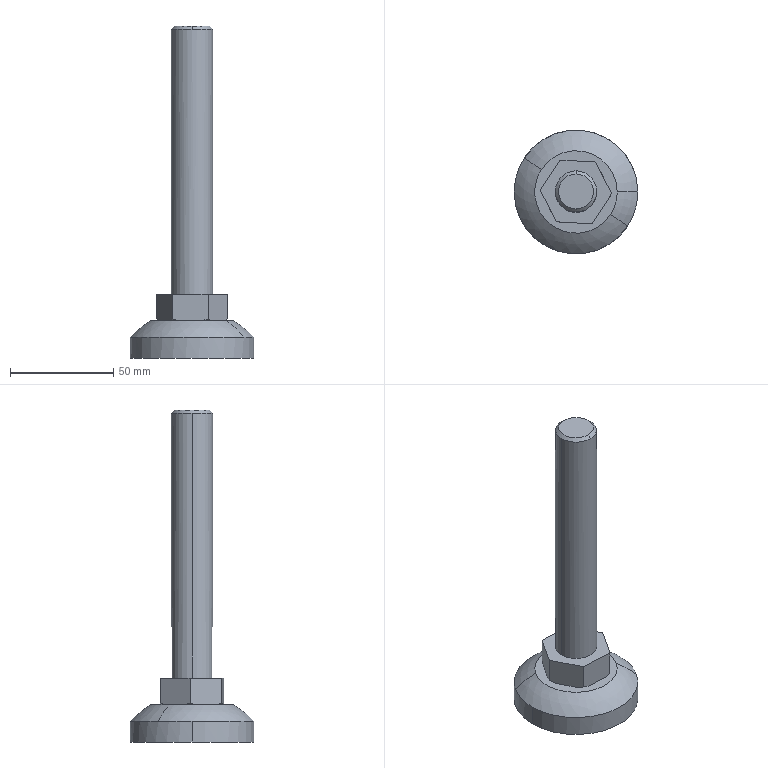Part | SolidWorks | features BaseBody 1 | 1 solid | 25 faces | box 60 x 60 x 161 mm | volume 95757 mm3 | plane 10 | cone 8 | cylinder 4 | torus 2 | spline 1 | commonest cylinder face diameters 20 x2 60 x2
STEP:
#1=CARTESIAN_POINT('',(-670.,1472.,-1500.534));
#2=VERTEX_POINT('',#1);
#3=CARTESIAN_POINT('',(-660.,1462.,-1500.534));
#4=VERTEX_POINT('',#3);
#5=CARTESIAN_POINT('',(-670.,1462.,-1500.534));
#6=DIRECTION('',(0.,0.,-1.));
#7=DIRECTION('',(-1.,0.,0.));
#8=AXIS2_PLACEMENT_3D('',#5,#6,#7);
#9=CIRCLE('',#8,10.);
#10=EDGE_CURVE('',#2,#4,#9,.T.);
#11=ORIENTED_EDGE('',*,*,#10,.T.);
#12=CARTESIAN_POINT('',(-660.,1462.,-1629.));
#13=VERTEX_POINT('',#12);
#14=CARTESIAN_POINT('',(-660.,1462.,-1499.));
#15=DIRECTION('',(0.,0.,-1.));
#16=VECTOR('',#15,1000.);
#17=LINE('',#14,#16);
#18=EDGE_CURVE('',#4,#13,#17,.T.);
#19=ORIENTED_EDGE('',*,*,#18,.T.);
#20=CARTESIAN_POINT('',(-680.,1462.,-1629.));
#21=VERTEX_POINT('',#20);
#22=CARTESIAN_POINT('',(-670.,1462.,-1629.));
#23=DIRECTION('',(0.,0.,1.));
#24=DIRECTION('',(-1.,0.,0.));
#25=AXIS2_PLACEMENT_3D('',#22,#23,#24);
#26=CIRCLE('',#25,10.);
#27=EDGE_CURVE('',#13,#21,#26,.T.);
#28=ORIENTED_EDGE('',*,*,#27,.T.);
#29=CARTESIAN_POINT('',(-680.,1462.,-1500.534));
#30=VERTEX_POINT('',#29);
#31=CARTESIAN_POINT('',(-680.,1462.,-1499.));
#32=DIRECTION('',(0.,0.,-1.));
#33=VECTOR('',#32,1000.);
#34=LINE('',#31,#33);
#35=EDGE_CURVE('',#30,#21,#34,.T.);
#36=ORIENTED_EDGE('',*,*,#35,.F.);
#37=CARTESIAN_POINT('',(-670.,1462.,-1500.534));
#38=DIRECTION('',(0.,0.,-1.));
#39=DIRECTION('',(-1.,0.,0.));
#40=AXIS2_PLACEMENT_3D('',#37,#38,#39);
#41=CIRCLE('',#40,10.);
#42=EDGE_CURVE('',#30,#2,#41,.T.);
#43=ORIENTED_EDGE('',*,*,#42,.T.);
#44=EDGE_LOOP('',(#11,#19,#28,#36,#43));
#45=FACE_OUTER_BOUND('',#44,.T.);
#46=CARTESIAN_POINT('',(-670.,1462.,-1499.));
#47=DIRECTION('',(0.,0.,-1.));
#48=DIRECTION('',(-1.,0.,0.));
#49=AXIS2_PLACEMENT_3D('',#46,#47,#48);
#50=CYLINDRICAL_SURFACE('',#49,10.);
#51=ADVANCED_FACE('',(#45),#50,.T.);
#52=CARTESIAN_POINT('',(-670.,1470.466,-1499.));
#53=VERTEX_POINT('',#52);
#54=CARTESIAN_POINT('',(-670.,1453.534,-1499.));
#55=VERTEX_POINT('',#54);
#56=CARTESIAN_POINT('',(-670.,1462.,-1499.));
#57=DIRECTION('',(0.,0.,-1.));
#58=DIRECTION('',(0.,1.,0.));
#59=AXIS2_PLACEMENT_3D('',#56,#57,#58);
#60=CIRCLE('',#59,8.466);
#61=EDGE_CURVE('',#53,#55,#60,.T.);
#62=ORIENTED_EDGE('',*,*,#61,.T.);
#63=CARTESIAN_POINT('',(-670.,1452.,-1500.534));
#64=VERTEX_POINT('',#63);
#65=CARTESIAN_POINT('',(-670.,1452.,-1500.533));
#66=DIRECTION('',(0.,-0.7071,-0.7071));
#67=VECTOR('',#66,1000.);
#68=LINE('',#65,#67);
#69=EDGE_CURVE('',#55,#64,#68,.T.);
#70=ORIENTED_EDGE('',*,*,#69,.T.);
#71=CARTESIAN_POINT('',(-670.,1462.,-1500.534));
#72=DIRECTION('',(0.,0.,-1.));
#73=DIRECTION('',(-1.,0.,0.));
#74=AXIS2_PLACEMENT_3D('',#71,#72,#73);
#75=CIRCLE('',#74,10.);
#76=EDGE_CURVE('',#4,#64,#75,.T.);
#77=ORIENTED_EDGE('',*,*,#76,.F.);
#78=ORIENTED_EDGE('',*,*,#10,.F.);
#79=CARTESIAN_POINT('',(-670.,1472.,-1500.533));
#80=DIRECTION('',(0.,0.7071,-0.7071));
#81=VECTOR('',#80,1000.);
#82=LINE('',#79,#81);
#83=EDGE_CURVE('',#53,#2,#82,.T.);
#84=ORIENTED_EDGE('',*,*,#83,.F.);
#85=EDGE_LOOP('',(#62,#70,#77,#78,#84));
#86=FACE_OUTER_BOUND('',#85,.T.);
#87=CARTESIAN_POINT('',(-670.,1462.,-1500.533));
#88=DIRECTION('',(0.,0.,-1.));
#89=DIRECTION('',(0.,1.,0.));
#90=AXIS2_PLACEMENT_3D('',#87,#88,#89);
#91=CONICAL_SURFACE('',#90,10.,0.7854);
#92=ADVANCED_FACE('',(#86),#91,.T.);
#93=CARTESIAN_POINT('',(-644.885,1445.592,-1650.));
#94=VERTEX_POINT('',#93);
#95=CARTESIAN_POINT('',(-640.,1462.,-1650.));
#96=VERTEX_POINT('',#95);
#97=CARTESIAN_POINT('',(-670.,1462.,-1650.));
#98=DIRECTION('',(0.,0.,1.));
#99=DIRECTION('',(0.8012,-0.5984,0.));
#100=AXIS2_PLACEMENT_3D('',#97,#98,#99);
#101=CIRCLE('',#100,30.);
#102=EDGE_CURVE('',#94,#96,#101,.T.);
#103=ORIENTED_EDGE('',*,*,#102,.T.);
#104=CARTESIAN_POINT('',(-650.,1462.,-1642.));
#105=VERTEX_POINT('',#104);
#106=CARTESIAN_POINT('',(-670.456,1462.,-1677.82));
#107=DIRECTION('',(0.,-1.,0.));
#108=DIRECTION('',(0.,0.,-1.));
#109=AXIS2_PLACEMENT_3D('',#106,#107,#108);
#110=CIRCLE('',#109,41.25);
#111=EDGE_CURVE('',#96,#105,#110,.T.);
#112=ORIENTED_EDGE('',*,*,#111,.T.);
#113=CARTESIAN_POINT('',(-653.257,1451.061,-1642.));
#114=VERTEX_POINT('',#113);
#115=CARTESIAN_POINT('',(-670.,1462.,-1642.));
#116=DIRECTION('',(0.,0.,-1.));
#117=DIRECTION('',(1.,0.,0.));
#118=AXIS2_PLACEMENT_3D('',#115,#116,#117);
#119=CIRCLE('',#118,20.);
#120=EDGE_CURVE('',#105,#114,#119,.T.);
#121=ORIENTED_EDGE('',*,*,#120,.T.);
#122=CARTESIAN_POINT('',(-670.382,1462.25,-1677.82));
#123=DIRECTION('',(0.5469,0.8372,0.));
#124=DIRECTION('',(0.6216,-0.4061,0.6698));
#125=AXIS2_PLACEMENT_3D('',#122,#123,#124);
#126=CIRCLE('',#125,41.25);
#127=EDGE_CURVE('',#114,#94,#126,.T.);
#128=ORIENTED_EDGE('',*,*,#127,.T.);
#129=EDGE_LOOP('',(#103,#112,#121,#128));
#130=FACE_OUTER_BOUND('',#129,.T.);
#131=CARTESIAN_POINT('',(-670.,1462.,-1677.82));
#132=DIRECTION('',(0.,0.,1.));
#133=DIRECTION('',(1.,0.,0.));
#134=AXIS2_PLACEMENT_3D('',#131,#132,#133);
#135=TOROIDAL_SURFACE('',#134,-0.4563,41.25);
#136=ADVANCED_FACE('',(#130),#135,.T.);
#137=CARTESIAN_POINT('',(-695.115,1478.408,-1650.));
#138=VERTEX_POINT('',#137);
#139=CARTESIAN_POINT('',(-670.,1462.,-1650.));
#140=DIRECTION('',(0.,0.,1.));
#141=DIRECTION('',(0.8012,-0.5984,0.));
#142=AXIS2_PLACEMENT_3D('',#139,#140,#141);
#143=CIRCLE('',#142,30.);
#144=EDGE_CURVE('',#96,#138,#143,.T.);
#145=ORIENTED_EDGE('',*,*,#144,.F.);
#146=CARTESIAN_POINT('',(-640.,1462.,-1660.));
#147=VERTEX_POINT('',#146);
#148=CARTESIAN_POINT('',(-640.,1462.,-1499.));
#149=DIRECTION('',(0.,0.,-1.));
#150=VECTOR('',#149,1000.);
#151=LINE('',#148,#150);
#152=EDGE_CURVE('',#96,#147,#151,.T.);
#153=ORIENTED_EDGE('',*,*,#152,.T.);
#154=CARTESIAN_POINT('',(-700.,1462.,-1660.));
#155=VERTEX_POINT('',#154);
#156=CARTESIAN_POINT('',(-670.,1462.,-1660.));
#157=DIRECTION('',(0.,0.,1.));
#158=DIRECTION('',(-1.,0.,0.));
#159=AXIS2_PLACEMENT_3D('',#156,#157,#158);
#160=CIRCLE('',#159,30.);
#161=EDGE_CURVE('',#147,#155,#160,.T.);
#162=ORIENTED_EDGE('',*,*,#161,.T.);
#163=CARTESIAN_POINT('',(-700.,1462.,-1650.));
#164=VERTEX_POINT('',#163);
#165=CARTESIAN_POINT('',(-700.,1462.,-1499.));
#166=DIRECTION('',(0.,0.,-1.));
#167=VECTOR('',#166,1000.);
#168=LINE('',#165,#167);
#169=EDGE_CURVE('',#164,#155,#168,.T.);
#170=ORIENTED_EDGE('',*,*,#169,.F.);
#171=CARTESIAN_POINT('',(-670.,1462.,-1650.));
#172=DIRECTION('',(0.,0.,1.));
#173=DIRECTION('',(-0.8012,0.5984,0.));
#174=AXIS2_PLACEMENT_3D('',#171,#172,#173);
#175=CIRCLE('',#174,30.);
#176=EDGE_CURVE('',#138,#164,#175,.T.);
#177=ORIENTED_EDGE('',*,*,#176,.F.);
#178=EDGE_LOOP('',(#145,#153,#162,#170,#177));
#179=FACE_OUTER_BOUND('',#178,.T.);
#180=CARTESIAN_POINT('',(-670.,1462.,-1499.));
#181=DIRECTION('',(0.,0.,-1.));
#182=DIRECTION('',(-1.,0.,0.));
#183=AXIS2_PLACEMENT_3D('',#180,#181,#182);
#184=CYLINDRICAL_SURFACE('',#183,30.);
#185=ADVANCED_FACE('',(#179),#184,.T.);
#186=ORIENTED_EDGE('',*,*,#18,.F.);
#187=ORIENTED_EDGE('',*,*,#76,.T.);
#188=CARTESIAN_POINT('',(-670.,1462.,-1500.534));
#189=DIRECTION('',(0.,0.,-1.));
#190=DIRECTION('',(-1.,0.,0.));
#191=AXIS2_PLACEMENT_3D('',#188,#189,#190);
#192=CIRCLE('',#191,10.);
#193=EDGE_CURVE('',#64,#30,#192,.T.);
#194=ORIENTED_EDGE('',*,*,#193,.T.);
#195=ORIENTED_EDGE('',*,*,#35,.T.);
#196=CARTESIAN_POINT('',(-670.,1462.,-1629.));
#197=DIRECTION('',(0.,0.,1.));
#198=DIRECTION('',(-1.,0.,0.));
#199=AXIS2_PLACEMENT_3D('',#196,#197,#198);
#200=CIRCLE('',#199,10.);
#201=EDGE_CURVE('',#21,#13,#200,.T.);
#202=ORIENTED_EDGE('',*,*,#201,.T.);
#203=EDGE_LOOP('',(#186,#187,#194,#195,#202));
#204=FACE_OUTER_BOUND('',#203,.T.);
#205=CARTESIAN_POINT('',(-670.,1462.,-1499.));
#206=DIRECTION('',(0.,0.,-1.));
#207=DIRECTION('',(-1.,0.,0.));
#208=AXIS2_PLACEMENT_3D('',#205,#206,#207);
#209=CYLINDRICAL_SURFACE('',#208,10.);
#210=ADVANCED_FACE('',(#204),#209,.T.);
#211=ORIENTED_EDGE('',*,*,#201,.F.);
#212=ORIENTED_EDGE('',*,*,#27,.F.);
#213=EDGE_LOOP('',(#211,#212));
#214=FACE_BOUND('',#213,.T.);
#215=CARTESIAN_POINT('',(-679.473,1447.5,-1629.));
#216=VERTEX_POINT('',#215);
#217=CARTESIAN_POINT('',(-687.294,1462.954,-1629.));
#218=VERTEX_POINT('',#217);
#219=CARTESIAN_POINT('',(-679.473,1447.5,-1629.));
#220=DIRECTION('',(-0.4515,0.8923,0.));
#221=VECTOR('',#220,1000.);
#222=LINE('',#219,#221);
#223=EDGE_CURVE('',#216,#218,#222,.T.);
#224=ORIENTED_EDGE('',*,*,#223,.F.);
#225=CARTESIAN_POINT('',(-662.179,1446.546,-1629.));
#226=VERTEX_POINT('',#225);
#227=CARTESIAN_POINT('',(-662.179,1446.546,-1629.));
#228=DIRECTION('',(-0.9985,0.05508,0.));
#229=VECTOR('',#228,1000.);
#230=LINE('',#227,#229);
#231=EDGE_CURVE('',#226,#216,#230,.T.);
#232=ORIENTED_EDGE('',*,*,#231,.F.);
#233=CARTESIAN_POINT('',(-652.706,1461.046,-1629.));
#234=VERTEX_POINT('',#233);
#235=CARTESIAN_POINT('',(-652.706,1461.046,-1629.));
#236=DIRECTION('',(-0.5469,-0.8372,0.));
#237=VECTOR('',#236,1000.);
#238=LINE('',#235,#237);
#239=EDGE_CURVE('',#234,#226,#238,.T.);
#240=ORIENTED_EDGE('',*,*,#239,.F.);
#241=CARTESIAN_POINT('',(-660.527,1476.5,-1629.));
#242=VERTEX_POINT('',#241);
#243=CARTESIAN_POINT('',(-660.527,1476.5,-1629.));
#244=DIRECTION('',(0.4515,-0.8923,0.));
#245=VECTOR('',#244,1000.);
#246=LINE('',#243,#245);
#247=EDGE_CURVE('',#242,#234,#246,.T.);
#248=ORIENTED_EDGE('',*,*,#247,.F.);
#249=CARTESIAN_POINT('',(-677.821,1477.454,-1629.));
#250=VERTEX_POINT('',#249);
#251=CARTESIAN_POINT('',(-677.821,1477.454,-1629.));
#252=DIRECTION('',(0.9985,-0.05508,0.));
#253=VECTOR('',#252,1000.);
#254=LINE('',#251,#253);
#255=EDGE_CURVE('',#250,#242,#254,.T.);
#256=ORIENTED_EDGE('',*,*,#255,.F.);
#257=CARTESIAN_POINT('',(-687.294,1462.954,-1629.));
#258=DIRECTION('',(0.5469,0.8372,0.));
#259=VECTOR('',#258,1000.);
#260=LINE('',#257,#259);
#261=EDGE_CURVE('',#218,#250,#260,.T.);
#262=ORIENTED_EDGE('',*,*,#261,.F.);
#263=EDGE_LOOP('',(#224,#232,#240,#248,#256,#262));
#264=FACE_OUTER_BOUND('',#263,.T.);
#265=CARTESIAN_POINT('',(-660.155,1477.069,-1629.));
#266=DIRECTION('',(0.,0.,-1.));
#267=DIRECTION('',(-1.,0.,0.));
#268=AXIS2_PLACEMENT_3D('',#265,#266,#267);
#269=PLANE('',#268);
#270=ADVANCED_FACE('',(#214,#264),#269,.F.);
#271=ORIENTED_EDGE('',*,*,#69,.F.);
#272=CARTESIAN_POINT('',(-670.,1462.,-1499.));
#273=DIRECTION('',(0.,0.,-1.));
#274=DIRECTION('',(0.,1.,0.));
#275=AXIS2_PLACEMENT_3D('',#272,#273,#274);
#276=CIRCLE('',#275,8.466);
#277=EDGE_CURVE('',#55,#53,#276,.T.);
#278=ORIENTED_EDGE('',*,*,#277,.T.);
#279=ORIENTED_EDGE('',*,*,#83,.T.);
#280=ORIENTED_EDGE('',*,*,#42,.F.);
#281=ORIENTED_EDGE('',*,*,#193,.F.);
#282=EDGE_LOOP('',(#271,#278,#279,#280,#281));
#283=FACE_OUTER_BOUND('',#282,.T.);
#284=CARTESIAN_POINT('',(-670.,1462.,-1500.533));
#285=DIRECTION('',(0.,0.,-1.));
#286=DIRECTION('',(0.,1.,0.));
#287=AXIS2_PLACEMENT_3D('',#284,#285,#286);
#288=CONICAL_SURFACE('',#287,10.,0.7854);
#289=ADVANCED_FACE('',(#283),#288,.T.);
#290=CARTESIAN_POINT('',(-677.821,1477.454,-1641.01));
#291=VERTEX_POINT('',#290);
#292=CARTESIAN_POINT('',(-677.821,1477.454,-1642.));
#293=DIRECTION('',(0.,0.,-1.));
#294=VECTOR('',#293,1000.);
#295=LINE('',#292,#294);
#296=EDGE_CURVE('',#250,#291,#295,.T.);
#297=ORIENTED_EDGE('',*,*,#296,.T.);
#298=CARTESIAN_POINT('',(-679.512,1474.865,-1642.));
#299=VERTEX_POINT('',#298);
#300=CARTESIAN_POINT('',(-677.821,1477.454,-1641.01));
#301=CARTESIAN_POINT('',(-678.376,1476.605,-1641.39));
#302=CARTESIAN_POINT('',(-678.939,1475.743,-1641.726));
#303=CARTESIAN_POINT('',(-679.512,1474.865,-1642.));
#304=B_SPLINE_CURVE_WITH_KNOTS('',3,(#300,#301,#302,#303),.UNSPECIFIED.,.F.,.F.,(4,4),(0.,0.003247),.UNSPECIFIED.);
#305=EDGE_CURVE('',#291,#299,#304,.T.);
#306=ORIENTED_EDGE('',*,*,#305,.T.);
#307=CARTESIAN_POINT('',(-685.603,1465.543,-1642.));
#308=VERTEX_POINT('',#307);
#309=CARTESIAN_POINT('',(-677.821,1477.454,-1642.));
#310=DIRECTION('',(-0.5469,-0.8372,0.));
#311=VECTOR('',#310,1000.);
#312=LINE('',#309,#311);
#313=EDGE_CURVE('',#299,#308,#312,.T.);
#314=ORIENTED_EDGE('',*,*,#313,.T.);
#315=CARTESIAN_POINT('',(-687.294,1462.954,-1641.01));
#316=VERTEX_POINT('',#315);
#317=CARTESIAN_POINT('',(-685.603,1465.543,-1642.));
#318=CARTESIAN_POINT('',(-686.176,1464.665,-1641.726));
#319=CARTESIAN_POINT('',(-686.739,1463.804,-1641.39));
#320=CARTESIAN_POINT('',(-687.294,1462.954,-1641.01));
#321=B_SPLINE_CURVE_WITH_KNOTS('',3,(#317,#318,#319,#320),.UNSPECIFIED.,.F.,.F.,(4,4),(0.,0.003247),.UNSPECIFIED.);
#322=EDGE_CURVE('',#308,#316,#321,.T.);
#323=ORIENTED_EDGE('',*,*,#322,.T.);
#324=CARTESIAN_POINT('',(-687.294,1462.954,-1642.));
#325=DIRECTION('',(0.,0.,1.));
#326=VECTOR('',#325,1000.);
#327=LINE('',#324,#326);
#328=EDGE_CURVE('',#316,#218,#327,.T.);
#329=ORIENTED_EDGE('',*,*,#328,.T.);
#330=ORIENTED_EDGE('',*,*,#261,.T.);
#331=EDGE_LOOP('',(#297,#306,#314,#323,#329,#330));
#332=FACE_OUTER_BOUND('',#331,.T.);
#333=CARTESIAN_POINT('',(-677.821,1477.454,-1642.));
#334=DIRECTION('',(-0.8372,0.5469,0.));
#335=DIRECTION('',(-0.5469,-0.8372,0.));
#336=AXIS2_PLACEMENT_3D('',#333,#334,#335);
#337=PLANE('',#336);
#338=ADVANCED_FACE('',(#332),#337,.T.);
#339=ORIENTED_EDGE('',*,*,#328,.F.);
#340=CARTESIAN_POINT('',(-685.898,1460.195,-1642.));
#341=VERTEX_POINT('',#340);
#342=CARTESIAN_POINT('',(-687.294,1462.954,-1641.01));
#343=CARTESIAN_POINT('',(-686.836,1462.049,-1641.39));
#344=CARTESIAN_POINT('',(-686.371,1461.131,-1641.726));
#345=CARTESIAN_POINT('',(-685.898,1460.195,-1642.));
#346=B_SPLINE_CURVE_WITH_KNOTS('',3,(#342,#343,#344,#345),.UNSPECIFIED.,.F.,.F.,(4,4),(0.,0.003247),.UNSPECIFIED.);
#347=EDGE_CURVE('',#316,#341,#346,.T.);
#348=ORIENTED_EDGE('',*,*,#347,.T.);
#349=CARTESIAN_POINT('',(-680.87,1450.259,-1642.));
#350=VERTEX_POINT('',#349);
#351=CARTESIAN_POINT('',(-687.294,1462.954,-1642.));
#352=DIRECTION('',(0.4515,-0.8923,0.));
#353=VECTOR('',#352,1000.);
#354=LINE('',#351,#353);
#355=EDGE_CURVE('',#341,#350,#354,.T.);
#356=ORIENTED_EDGE('',*,*,#355,.T.);
#357=CARTESIAN_POINT('',(-679.473,1447.5,-1641.01));
#358=VERTEX_POINT('',#357);
#359=CARTESIAN_POINT('',(-680.87,1450.259,-1642.));
#360=CARTESIAN_POINT('',(-680.396,1449.323,-1641.726));
#361=CARTESIAN_POINT('',(-679.932,1448.405,-1641.39));
#362=CARTESIAN_POINT('',(-679.473,1447.5,-1641.01));
#363=B_SPLINE_CURVE_WITH_KNOTS('',3,(#359,#360,#361,#362),.UNSPECIFIED.,.F.,.F.,(4,4),(0.,0.003247),.UNSPECIFIED.);
#364=EDGE_CURVE('',#350,#358,#363,.T.);
#365=ORIENTED_EDGE('',*,*,#364,.T.);
#366=CARTESIAN_POINT('',(-679.473,1447.5,-1642.));
#367=DIRECTION('',(0.,0.,1.));
#368=VECTOR('',#367,1000.);
#369=LINE('',#366,#368);
#370=EDGE_CURVE('',#358,#216,#369,.T.);
#371=ORIENTED_EDGE('',*,*,#370,.T.);
#372=ORIENTED_EDGE('',*,*,#223,.T.);
#373=EDGE_LOOP('',(#339,#348,#356,#365,#371,#372));
#374=FACE_OUTER_BOUND('',#373,.T.);
#375=CARTESIAN_POINT('',(-687.294,1462.954,-1642.));
#376=DIRECTION('',(-0.8923,-0.4515,0.));
#377=DIRECTION('',(0.4515,-0.8923,0.));
#378=AXIS2_PLACEMENT_3D('',#375,#376,#377);
#379=PLANE('',#378);
#380=ADVANCED_FACE('',(#374),#379,.T.);
#381=ORIENTED_EDGE('',*,*,#370,.F.);
#382=CARTESIAN_POINT('',(-676.386,1447.329,-1642.));
#383=VERTEX_POINT('',#382);
#384=CARTESIAN_POINT('',(-679.473,1447.5,-1641.01));
#385=CARTESIAN_POINT('',(-678.46,1447.444,-1641.39));
#386=CARTESIAN_POINT('',(-677.433,1447.387,-1641.726));
#387=CARTESIAN_POINT('',(-676.386,1447.329,-1642.));
#388=B_SPLINE_CURVE_WITH_KNOTS('',3,(#384,#385,#386,#387),.UNSPECIFIED.,.F.,.F.,(4,4),(0.,0.003247),.UNSPECIFIED.);
#389=EDGE_CURVE('',#358,#383,#388,.T.);
#390=ORIENTED_EDGE('',*,*,#389,.T.);
#391=CARTESIAN_POINT('',(-665.267,1446.716,-1642.));
#392=VERTEX_POINT('',#391);
#393=CARTESIAN_POINT('',(-679.473,1447.5,-1642.));
#394=DIRECTION('',(0.9985,-0.05508,0.));
#395=VECTOR('',#394,1000.);
#396=LINE('',#393,#395);
#397=EDGE_CURVE('',#383,#392,#396,.T.);
#398=ORIENTED_EDGE('',*,*,#397,.T.);
#399=CARTESIAN_POINT('',(-662.179,1446.546,-1641.01));
#400=VERTEX_POINT('',#399);
#401=CARTESIAN_POINT('',(-665.267,1446.716,-1642.));
#402=CARTESIAN_POINT('',(-664.22,1446.658,-1641.726));
#403=CARTESIAN_POINT('',(-663.192,1446.602,-1641.39));
#404=CARTESIAN_POINT('',(-662.179,1446.546,-1641.01));
#405=B_SPLINE_CURVE_WITH_KNOTS('',3,(#401,#402,#403,#404),.UNSPECIFIED.,.F.,.F.,(4,4),(0.,0.003247),.UNSPECIFIED.);
#406=EDGE_CURVE('',#392,#400,#405,.T.);
#407=ORIENTED_EDGE('',*,*,#406,.T.);
#408=CARTESIAN_POINT('',(-662.179,1446.546,-1642.));
#409=DIRECTION('',(0.,0.,1.));
#410=VECTOR('',#409,1000.);
#411=LINE('',#408,#410);
#412=EDGE_CURVE('',#400,#226,#411,.T.);
#413=ORIENTED_EDGE('',*,*,#412,.T.);
#414=ORIENTED_EDGE('',*,*,#231,.T.);
#415=EDGE_LOOP('',(#381,#390,#398,#407,#413,#414));
#416=FACE_OUTER_BOUND('',#415,.T.);
#417=CARTESIAN_POINT('',(-679.473,1447.5,-1642.));
#418=DIRECTION('',(-0.05508,-0.9985,0.));
#419=DIRECTION('',(0.9985,-0.05508,0.));
#420=AXIS2_PLACEMENT_3D('',#417,#418,#419);
#421=PLANE('',#420);
#422=ADVANCED_FACE('',(#416),#421,.T.);
#423=ORIENTED_EDGE('',*,*,#412,.F.);
#424=CARTESIAN_POINT('',(-660.488,1449.135,-1642.));
#425=VERTEX_POINT('',#424);
#426=CARTESIAN_POINT('',(-662.179,1446.546,-1641.01));
#427=CARTESIAN_POINT('',(-661.624,1447.395,-1641.39));
#428=CARTESIAN_POINT('',(-661.061,1448.257,-1641.726));
#429=CARTESIAN_POINT('',(-660.488,1449.135,-1642.));
#430=B_SPLINE_CURVE_WITH_KNOTS('',3,(#426,#427,#428,#429),.UNSPECIFIED.,.F.,.F.,(4,4),(0.,0.003247),.UNSPECIFIED.);
#431=EDGE_CURVE('',#400,#425,#430,.T.);
#432=ORIENTED_EDGE('',*,*,#431,.T.);
#433=CARTESIAN_POINT('',(-654.397,1458.457,-1642.));
#434=VERTEX_POINT('',#433);
#435=CARTESIAN_POINT('',(-662.179,1446.546,-1642.));
#436=DIRECTION('',(0.5469,0.8372,0.));
#437=VECTOR('',#436,1000.);
#438=LINE('',#435,#437);
#439=EDGE_CURVE('',#425,#434,#438,.T.);
#440=ORIENTED_EDGE('',*,*,#439,.T.);
#441=CARTESIAN_POINT('',(-652.706,1461.046,-1641.01));
#442=VERTEX_POINT('',#441);
#443=CARTESIAN_POINT('',(-654.397,1458.457,-1642.));
#444=CARTESIAN_POINT('',(-653.824,1459.335,-1641.726));
#445=CARTESIAN_POINT('',(-653.261,1460.196,-1641.39));
#446=CARTESIAN_POINT('',(-652.706,1461.046,-1641.01));
#447=B_SPLINE_CURVE_WITH_KNOTS('',3,(#443,#444,#445,#446),.UNSPECIFIED.,.F.,.F.,(4,4),(0.,0.003247),.UNSPECIFIED.);
#448=EDGE_CURVE('',#434,#442,#447,.T.);
#449=ORIENTED_EDGE('',*,*,#448,.T.);
#450=CARTESIAN_POINT('',(-652.706,1461.046,-1642.));
#451=DIRECTION('',(0.,0.,1.));
#452=VECTOR('',#451,1000.);
#453=LINE('',#450,#452);
#454=EDGE_CURVE('',#442,#234,#453,.T.);
#455=ORIENTED_EDGE('',*,*,#454,.T.);
#456=ORIENTED_EDGE('',*,*,#239,.T.);
#457=EDGE_LOOP('',(#423,#432,#440,#449,#455,#456));
#458=FACE_OUTER_BOUND('',#457,.T.);
#459=CARTESIAN_POINT('',(-662.179,1446.546,-1642.));
#460=DIRECTION('',(0.8372,-0.5469,0.));
#461=DIRECTION('',(0.5469,0.8372,0.));
#462=AXIS2_PLACEMENT_3D('',#459,#460,#461);
#463=PLANE('',#462);
#464=ADVANCED_FACE('',(#458),#463,.T.);
#465=ORIENTED_EDGE('',*,*,#454,.F.);
#466=CARTESIAN_POINT('',(-654.102,1463.805,-1642.));
#467=VERTEX_POINT('',#466);
#468=CARTESIAN_POINT('',(-652.706,1461.046,-1641.01));
#469=CARTESIAN_POINT('',(-653.164,1461.951,-1641.39));
#470=CARTESIAN_POINT('',(-653.629,1462.869,-1641.726));
#471=CARTESIAN_POINT('',(-654.102,1463.805,-1642.));
#472=B_SPLINE_CURVE_WITH_KNOTS('',3,(#468,#469,#470,#471),.UNSPECIFIED.,.F.,.F.,(4,4),(0.,0.003247),.UNSPECIFIED.);
#473=EDGE_CURVE('',#442,#467,#472,.T.);
#474=ORIENTED_EDGE('',*,*,#473,.T.);
#475=CARTESIAN_POINT('',(-659.13,1473.741,-1642.));
#476=VERTEX_POINT('',#475);
#477=CARTESIAN_POINT('',(-652.706,1461.046,-1642.));
#478=DIRECTION('',(-0.4515,0.8923,0.));
#479=VECTOR('',#478,1000.);
#480=LINE('',#477,#479);
#481=EDGE_CURVE('',#467,#476,#480,.T.);
#482=ORIENTED_EDGE('',*,*,#481,.T.);
#483=CARTESIAN_POINT('',(-660.527,1476.5,-1641.01));
#484=VERTEX_POINT('',#483);
#485=CARTESIAN_POINT('',(-659.13,1473.741,-1642.));
#486=CARTESIAN_POINT('',(-659.604,1474.677,-1641.726));
#487=CARTESIAN_POINT('',(-660.068,1475.595,-1641.39));
#488=CARTESIAN_POINT('',(-660.527,1476.5,-1641.01));
#489=B_SPLINE_CURVE_WITH_KNOTS('',3,(#485,#486,#487,#488),.UNSPECIFIED.,.F.,.F.,(4,4),(0.,0.003247),.UNSPECIFIED.);
#490=EDGE_CURVE('',#476,#484,#489,.T.);
#491=ORIENTED_EDGE('',*,*,#490,.T.);
#492=CARTESIAN_POINT('',(-660.527,1476.5,-1642.));
#493=DIRECTION('',(0.,0.,1.));
#494=VECTOR('',#493,1000.);
#495=LINE('',#492,#494);
#496=EDGE_CURVE('',#484,#242,#495,.T.);
#497=ORIENTED_EDGE('',*,*,#496,.T.);
#498=ORIENTED_EDGE('',*,*,#247,.T.);
#499=EDGE_LOOP('',(#465,#474,#482,#491,#497,#498));
#500=FACE_OUTER_BOUND('',#499,.T.);
#501=CARTESIAN_POINT('',(-652.706,1461.046,-1642.));
#502=DIRECTION('',(0.8923,0.4515,0.));
#503=DIRECTION('',(-0.4515,0.8923,0.));
#504=AXIS2_PLACEMENT_3D('',#501,#502,#503);
#505=PLANE('',#504);
#506=ADVANCED_FACE('',(#500),#505,.T.);
#507=ORIENTED_EDGE('',*,*,#496,.F.);
#508=CARTESIAN_POINT('',(-663.614,1476.671,-1642.));
#509=VERTEX_POINT('',#508);
#510=CARTESIAN_POINT('',(-660.527,1476.5,-1641.01));
#511=CARTESIAN_POINT('',(-661.54,1476.556,-1641.39));
#512=CARTESIAN_POINT('',(-662.567,1476.613,-1641.726));
#513=CARTESIAN_POINT('',(-663.614,1476.671,-1642.));
#514=B_SPLINE_CURVE_WITH_KNOTS('',3,(#510,#511,#512,#513),.UNSPECIFIED.,.F.,.F.,(4,4),(0.,0.003247),.UNSPECIFIED.);
#515=EDGE_CURVE('',#484,#509,#514,.T.);
#516=ORIENTED_EDGE('',*,*,#515,.T.);
#517=CARTESIAN_POINT('',(-674.733,1477.284,-1642.));
#518=VERTEX_POINT('',#517);
#519=CARTESIAN_POINT('',(-660.527,1476.5,-1642.));
#520=DIRECTION('',(-0.9985,0.05508,0.));
#521=VECTOR('',#520,1000.);
#522=LINE('',#519,#521);
#523=EDGE_CURVE('',#509,#518,#522,.T.);
#524=ORIENTED_EDGE('',*,*,#523,.T.);
#525=CARTESIAN_POINT('',(-674.733,1477.284,-1642.));
#526=CARTESIAN_POINT('',(-675.78,1477.342,-1641.726));
#527=CARTESIAN_POINT('',(-676.808,1477.398,-1641.39));
#528=CARTESIAN_POINT('',(-677.821,1477.454,-1641.01));
#529=B_SPLINE_CURVE_WITH_KNOTS('',3,(#525,#526,#527,#528),.UNSPECIFIED.,.F.,.F.,(4,4),(0.,0.003247),.UNSPECIFIED.);
#530=EDGE_CURVE('',#518,#291,#529,.T.);
#531=ORIENTED_EDGE('',*,*,#530,.T.);
#532=ORIENTED_EDGE('',*,*,#296,.F.);
#533=ORIENTED_EDGE('',*,*,#255,.T.);
#534=EDGE_LOOP('',(#507,#516,#524,#531,#532,#533));
#535=FACE_OUTER_BOUND('',#534,.T.);
#536=CARTESIAN_POINT('',(-660.527,1476.5,-1642.));
#537=DIRECTION('',(0.05508,0.9985,0.));
#538=DIRECTION('',(-0.9985,0.05508,0.));
#539=AXIS2_PLACEMENT_3D('',#536,#537,#538);
#540=PLANE('',#539);
#541=ADVANCED_FACE('',(#535),#540,.T.);
#542=ORIENTED_EDGE('',*,*,#61,.F.);
#543=ORIENTED_EDGE('',*,*,#277,.F.);
#544=EDGE_LOOP('',(#542,#543));
#545=FACE_OUTER_BOUND('',#544,.T.);
#546=CARTESIAN_POINT('',(-665.369,1469.088,-1499.));
#547=DIRECTION('',(0.,0.,-1.));
#548=DIRECTION('',(-1.,0.,0.));
#549=AXIS2_PLACEMENT_3D('',#546,#547,#548);
#550=PLANE('',#549);
#551=ADVANCED_FACE('',(#545),#550,.F.);
#552=ORIENTED_EDGE('',*,*,#305,.F.);
#553=ORIENTED_EDGE('',*,*,#530,.F.);
#554=CARTESIAN_POINT('',(-670.,1462.,-1642.));
#555=DIRECTION('',(0.,0.,1.));
#556=DIRECTION('',(0.,-1.,0.));
#557=AXIS2_PLACEMENT_3D('',#554,#555,#556);
#558=CIRCLE('',#557,16.);
#559=EDGE_CURVE('',#518,#299,#558,.T.);
#560=ORIENTED_EDGE('',*,*,#559,.T.);
#561=EDGE_LOOP('',(#552,#553,#560));
#562=FACE_OUTER_BOUND('',#561,.T.);
#563=CARTESIAN_POINT('',(-670.,1462.,-1641.004));
#564=DIRECTION('',(0.,0.,1.));
#565=DIRECTION('',(0.,-1.,0.));
#566=AXIS2_PLACEMENT_3D('',#563,#564,#565);
#567=CONICAL_SURFACE('',#566,17.328,0.9273);
#568=ADVANCED_FACE('',(#562),#567,.T.);
#569=CARTESIAN_POINT('',(-670.,1462.,-1642.));
#570=DIRECTION('',(0.,0.,1.));
#571=DIRECTION('',(0.,-1.,0.));
#572=AXIS2_PLACEMENT_3D('',#569,#570,#571);
#573=CIRCLE('',#572,16.);
#574=EDGE_CURVE('',#308,#341,#573,.T.);
#575=ORIENTED_EDGE('',*,*,#574,.T.);
#576=ORIENTED_EDGE('',*,*,#347,.F.);
#577=ORIENTED_EDGE('',*,*,#322,.F.);
#578=EDGE_LOOP('',(#575,#576,#577));
#579=FACE_OUTER_BOUND('',#578,.T.);
#580=CARTESIAN_POINT('',(-670.,1462.,-1641.004));
#581=DIRECTION('',(0.,0.,1.));
#582=DIRECTION('',(0.,-1.,0.));
#583=AXIS2_PLACEMENT_3D('',#580,#581,#582);
#584=CONICAL_SURFACE('',#583,17.328,0.9273);
#585=ADVANCED_FACE('',(#579),#584,.T.);
#586=CARTESIAN_POINT('',(-670.,1462.,-1642.));
#587=DIRECTION('',(0.,0.,1.));
#588=DIRECTION('',(0.,-1.,0.));
#589=AXIS2_PLACEMENT_3D('',#586,#587,#588);
#590=CIRCLE('',#589,16.);
#591=EDGE_CURVE('',#476,#509,#590,.T.);
#592=ORIENTED_EDGE('',*,*,#591,.F.);
#593=ORIENTED_EDGE('',*,*,#481,.F.);
#594=CARTESIAN_POINT('',(-670.,1462.,-1642.));
#595=DIRECTION('',(0.,0.,1.));
#596=DIRECTION('',(0.,-1.,0.));
#597=AXIS2_PLACEMENT_3D('',#594,#595,#596);
#598=CIRCLE('',#597,16.);
#599=EDGE_CURVE('',#434,#467,#598,.T.);
#600=ORIENTED_EDGE('',*,*,#599,.F.);
#601=ORIENTED_EDGE('',*,*,#439,.F.);
#602=CARTESIAN_POINT('',(-670.,1462.,-1642.));
#603=DIRECTION('',(0.,0.,1.));
#604=DIRECTION('',(0.,-1.,0.));
#605=AXIS2_PLACEMENT_3D('',#602,#603,#604);
#606=CIRCLE('',#605,16.);
#607=EDGE_CURVE('',#392,#425,#606,.T.);
#608=ORIENTED_EDGE('',*,*,#607,.F.);
#609=ORIENTED_EDGE('',*,*,#397,.F.);
#610=CARTESIAN_POINT('',(-670.,1462.,-1642.));
#611=DIRECTION('',(0.,0.,1.));
#612=DIRECTION('',(1.,0.,0.));
#613=AXIS2_PLACEMENT_3D('',#610,#611,#612);
#614=CIRCLE('',#613,16.);
#615=EDGE_CURVE('',#350,#383,#614,.T.);
#616=ORIENTED_EDGE('',*,*,#615,.F.);
#617=ORIENTED_EDGE('',*,*,#355,.F.);
#618=ORIENTED_EDGE('',*,*,#574,.F.);
#619=ORIENTED_EDGE('',*,*,#313,.F.);
#620=ORIENTED_EDGE('',*,*,#559,.F.);
#621=ORIENTED_EDGE('',*,*,#523,.F.);
#622=EDGE_LOOP('',(#592,#593,#600,#601,#608,#609,#616,#617,#618,#619,#620,#621));
#623=FACE_BOUND('',#622,.T.);
#624=CARTESIAN_POINT('',(-686.743,1472.939,-1642.));
#625=VERTEX_POINT('',#624);
#626=CARTESIAN_POINT('',(-653.257,1451.061,-1642.));
#627=CARTESIAN_POINT('',(-659.699,1441.2,-1642.));
#628=CARTESIAN_POINT('',(-671.184,1438.883,-1642.));
#629=CARTESIAN_POINT('',(-680.939,1445.257,-1642.));
#630=CARTESIAN_POINT('',(-690.694,1451.63,-1642.));
#631=CARTESIAN_POINT('',(-693.186,1463.078,-1642.));
#632=CARTESIAN_POINT('',(-686.743,1472.939,-1642.));
#633=(BOUNDED_CURVE()B_SPLINE_CURVE(3,(#626,#627,#628,#629,#630,#631,#632),.UNSPECIFIED.,.F.,.F.)B_SPLINE_CURVE_WITH_KNOTS((4,3,4),(0.,0.03112,0.06224),.UNSPECIFIED.)CURVE()GEOMETRIC_REPRESENTATION_ITEM()RATIONAL_B_SPLINE_CURVE((1.164,0.9438,0.954,1.195,0.954,0.9438,1.164))REPRESENTATION_ITEM(''));
#634=EDGE_CURVE('',#114,#625,#633,.T.);
#635=ORIENTED_EDGE('',*,*,#634,.F.);
#636=ORIENTED_EDGE('',*,*,#120,.F.);
#637=CARTESIAN_POINT('',(-670.,1462.,-1642.));
#638=DIRECTION('',(0.,0.,-1.));
#639=DIRECTION('',(1.,0.,0.));
#640=AXIS2_PLACEMENT_3D('',#637,#638,#639);
#641=CIRCLE('',#640,20.);
#642=EDGE_CURVE('',#625,#105,#641,.T.);
#643=ORIENTED_EDGE('',*,*,#642,.F.);
#644=EDGE_LOOP('',(#635,#636,#643));
#645=FACE_OUTER_BOUND('',#644,.T.);
#646=CARTESIAN_POINT('',(-659.061,1478.743,-1642.));
#647=DIRECTION('',(0.,0.,-1.));
#648=DIRECTION('',(-1.,0.,0.));
#649=AXIS2_PLACEMENT_3D('',#646,#647,#648);
#650=PLANE('',#649);
#651=ADVANCED_FACE('',(#623,#645),#650,.F.);
#652=ORIENTED_EDGE('',*,*,#615,.T.);
#653=ORIENTED_EDGE('',*,*,#389,.F.);
#654=ORIENTED_EDGE('',*,*,#364,.F.);
#655=EDGE_LOOP('',(#652,#653,#654));
#656=FACE_OUTER_BOUND('',#655,.T.);
#657=CARTESIAN_POINT('',(-670.,1462.,-1641.004));
#658=DIRECTION('',(0.,0.,1.));
#659=DIRECTION('',(1.,0.,0.));
#660=AXIS2_PLACEMENT_3D('',#657,#658,#659);
#661=CONICAL_SURFACE('',#660,17.328,0.9273);
#662=ADVANCED_FACE('',(#656),#661,.T.);
#663=ORIENTED_EDGE('',*,*,#607,.T.);
#664=ORIENTED_EDGE('',*,*,#431,.F.);
#665=ORIENTED_EDGE('',*,*,#406,.F.);
#666=EDGE_LOOP('',(#663,#664,#665));
#667=FACE_OUTER_BOUND('',#666,.T.);
#668=CARTESIAN_POINT('',(-670.,1462.,-1641.004));
#669=DIRECTION('',(0.,0.,1.));
#670=DIRECTION('',(0.,-1.,0.));
#671=AXIS2_PLACEMENT_3D('',#668,#669,#670);
#672=CONICAL_SURFACE('',#671,17.328,0.9273);
#673=ADVANCED_FACE('',(#667),#672,.T.);
#674=ORIENTED_EDGE('',*,*,#599,.T.);
#675=ORIENTED_EDGE('',*,*,#473,.F.);
#676=ORIENTED_EDGE('',*,*,#448,.F.);
#677=EDGE_LOOP('',(#674,#675,#676));
#678=FACE_OUTER_BOUND('',#677,.T.);
#679=CARTESIAN_POINT('',(-670.,1462.,-1641.004));
#680=DIRECTION('',(0.,0.,1.));
#681=DIRECTION('',(0.,-1.,0.));
#682=AXIS2_PLACEMENT_3D('',#679,#680,#681);
#683=CONICAL_SURFACE('',#682,17.328,0.9273);
#684=ADVANCED_FACE('',(#678),#683,.T.);
#685=ORIENTED_EDGE('',*,*,#591,.T.);
#686=ORIENTED_EDGE('',*,*,#515,.F.);
#687=ORIENTED_EDGE('',*,*,#490,.F.);
#688=EDGE_LOOP('',(#685,#686,#687));
#689=FACE_OUTER_BOUND('',#688,.T.);
#690=CARTESIAN_POINT('',(-670.,1462.,-1641.004));
#691=DIRECTION('',(0.,0.,1.));
#692=DIRECTION('',(0.,-1.,0.));
#693=AXIS2_PLACEMENT_3D('',#690,#691,#692);
#694=CONICAL_SURFACE('',#693,17.328,0.9273);
#695=ADVANCED_FACE('',(#689),#694,.T.);
#696=ORIENTED_EDGE('',*,*,#111,.F.);
#697=ORIENTED_EDGE('',*,*,#144,.T.);
#698=CARTESIAN_POINT('',(-669.618,1461.75,-1677.82));
#699=DIRECTION('',(0.5469,0.8372,0.));
#700=DIRECTION('',(-0.6216,0.4061,0.6698));
#701=AXIS2_PLACEMENT_3D('',#698,#699,#700);
#702=CIRCLE('',#701,41.25);
#703=EDGE_CURVE('',#138,#625,#702,.T.);
#704=ORIENTED_EDGE('',*,*,#703,.T.);
#705=ORIENTED_EDGE('',*,*,#642,.T.);
#706=EDGE_LOOP('',(#696,#697,#704,#705));
#707=FACE_OUTER_BOUND('',#706,.T.);
#708=CARTESIAN_POINT('',(-670.,1462.,-1677.82));
#709=DIRECTION('',(0.,0.,1.));
#710=DIRECTION('',(1.,0.,0.));
#711=AXIS2_PLACEMENT_3D('',#708,#709,#710);
#712=TOROIDAL_SURFACE('',#711,-0.4563,41.25);
#713=ADVANCED_FACE('',(#707),#712,.T.);
#714=ORIENTED_EDGE('',*,*,#703,.F.);
#715=ORIENTED_EDGE('',*,*,#176,.T.);
#716=CARTESIAN_POINT('',(-670.,1462.,-1650.));
#717=DIRECTION('',(0.,0.,1.));
#718=DIRECTION('',(-0.8012,0.5984,0.));
#719=AXIS2_PLACEMENT_3D('',#716,#717,#718);
#720=CIRCLE('',#719,30.);
#721=EDGE_CURVE('',#164,#94,#720,.T.);
#722=ORIENTED_EDGE('',*,*,#721,.T.);
#723=ORIENTED_EDGE('',*,*,#127,.F.);
#724=ORIENTED_EDGE('',*,*,#634,.T.);
#725=EDGE_LOOP('',(#714,#715,#722,#723,#724));
#726=FACE_OUTER_BOUND('',#725,.T.);
#727=CARTESIAN_POINT('',(-694.174,1480.056,-1650.19));
#728=CARTESIAN_POINT('',(-691.771,1478.262,-1646.866));
#729=CARTESIAN_POINT('',(-688.97,1476.169,-1644.069));
#730=CARTESIAN_POINT('',(-685.844,1473.834,-1641.873));
#731=CARTESIAN_POINT('',(-705.286,1465.18,-1650.19));
#732=CARTESIAN_POINT('',(-701.778,1464.864,-1646.866));
#733=CARTESIAN_POINT('',(-697.69,1464.495,-1644.069));
#734=CARTESIAN_POINT('',(-693.127,1464.084,-1641.873));
#735=CARTESIAN_POINT('',(-702.048,1446.896,-1650.19));
#736=CARTESIAN_POINT('',(-698.862,1448.397,-1646.866));
#737=CARTESIAN_POINT('',(-695.149,1450.147,-1644.069));
#738=CARTESIAN_POINT('',(-691.005,1452.101,-1641.873));
#739=CARTESIAN_POINT('',(-686.503,1436.74,-1650.19));
#740=CARTESIAN_POINT('',(-684.863,1439.251,-1646.866));
#741=CARTESIAN_POINT('',(-682.95,1442.178,-1644.069));
#742=CARTESIAN_POINT('',(-680.816,1445.444,-1641.873));
#743=CARTESIAN_POINT('',(-670.958,1426.584,-1650.19));
#744=CARTESIAN_POINT('',(-670.863,1430.104,-1646.866));
#745=CARTESIAN_POINT('',(-670.752,1434.208,-1644.069));
#746=CARTESIAN_POINT('',(-670.628,1438.788,-1641.873));
#747=CARTESIAN_POINT('',(-652.914,1430.964,-1650.19));
#748=CARTESIAN_POINT('',(-654.612,1434.049,-1646.866));
#749=CARTESIAN_POINT('',(-656.592,1437.645,-1644.069));
#750=CARTESIAN_POINT('',(-658.801,1441.658,-1641.873));
#751=CARTESIAN_POINT('',(-643.754,1447.116,-1650.19));
#752=CARTESIAN_POINT('',(-646.363,1448.595,-1646.866));
#753=CARTESIAN_POINT('',(-649.404,1450.32,-1644.069));
#754=CARTESIAN_POINT('',(-652.798,1452.245,-1641.873));
#755=(BOUNDED_SURFACE()B_SPLINE_SURFACE(3,3,((#727,#728,#729,#730),(#731,#732,#733,#734),(#735,#736,#737,#738),(#739,#740,#741,#742),(#743,#744,#745,#746),(#747,#748,#749,#750),(#751,#752,#753,#754)),.UNSPECIFIED.,.F.,.F.,.F.)B_SPLINE_SURFACE_WITH_KNOTS((4,3,4),(4,4),(0.,1.,2.),(0.,1.),.UNSPECIFIED.)GEOMETRIC_REPRESENTATION_ITEM()RATIONAL_B_SPLINE_SURFACE(((1.195,1.185,1.185,1.195),(0.9438,0.9355,0.9355,0.9438),(0.9438,0.9355,0.9355,0.9438),(1.195,1.185,1.185,1.195),(0.9438,0.9355,0.9355,0.9438),(0.9438,0.9355,0.9355,0.9438),(1.195,1.185,1.185,1.195)))REPRESENTATION_ITEM('')SURFACE());
#756=ADVANCED_FACE('',(#726),#755,.T.);
#757=ORIENTED_EDGE('',*,*,#152,.F.);
#758=ORIENTED_EDGE('',*,*,#102,.F.);
#759=ORIENTED_EDGE('',*,*,#721,.F.);
#760=ORIENTED_EDGE('',*,*,#169,.T.);
#761=CARTESIAN_POINT('',(-670.,1462.,-1660.));
#762=DIRECTION('',(0.,0.,1.));
#763=DIRECTION('',(-1.,0.,0.));
#764=AXIS2_PLACEMENT_3D('',#761,#762,#763);
#765=CIRCLE('',#764,30.);
#766=EDGE_CURVE('',#155,#147,#765,.T.);
#767=ORIENTED_EDGE('',*,*,#766,.T.);
#768=EDGE_LOOP('',(#757,#758,#759,#760,#767));
#769=FACE_OUTER_BOUND('',#768,.T.);
#770=CARTESIAN_POINT('',(-670.,1462.,-1499.));
#771=DIRECTION('',(0.,0.,-1.));
#772=DIRECTION('',(-1.,0.,0.));
#773=AXIS2_PLACEMENT_3D('',#770,#771,#772);
#774=CYLINDRICAL_SURFACE('',#773,30.);
#775=ADVANCED_FACE('',(#769),#774,.T.);
#776=ORIENTED_EDGE('',*,*,#766,.F.);
#777=ORIENTED_EDGE('',*,*,#161,.F.);
#778=EDGE_LOOP('',(#776,#777));
#779=FACE_OUTER_BOUND('',#778,.T.);
#780=CARTESIAN_POINT('',(-670.,1462.,-1660.));
#781=DIRECTION('',(0.,0.,1.));
#782=DIRECTION('',(1.,0.,0.));
#783=AXIS2_PLACEMENT_3D('',#780,#781,#782);
#784=PLANE('',#783);
#785=ADVANCED_FACE('',(#779),#784,.F.);
#786=CLOSED_SHELL('',(#51,#92,#136,#185,#210,#270,#289,#338,#380,#422,#464,#506,#541,#551,#568,#585,#651,#662,#673,#684,#695,#713,#756,#775,#785));
#787=MANIFOLD_SOLID_BREP('',#786);
#788=CARTESIAN_POINT('',(0.,0.,0.));
#789=DIRECTION('',(0.,0.,1.));
#790=DIRECTION('',(1.,0.,0.));
#791=AXIS2_PLACEMENT_3D('',#788,#789,#790);
#792=(LENGTH_UNIT()NAMED_UNIT(*)SI_UNIT(.MILLI.,.METRE.));
#793=UNCERTAINTY_MEASURE_WITH_UNIT(LENGTH_MEASURE(0.00001),#792,'','');
#794=(NAMED_UNIT(*)PLANE_ANGLE_UNIT()SI_UNIT($,.RADIAN.));
#795=(NAMED_UNIT(*)SI_UNIT($,.STERADIAN.)SOLID_ANGLE_UNIT());
#796=(GEOMETRIC_REPRESENTATION_CONTEXT(3)GLOBAL_UNCERTAINTY_ASSIGNED_CONTEXT((#793))GLOBAL_UNIT_ASSIGNED_CONTEXT((#792,#794,#795))REPRESENTATION_CONTEXT('',''));
#797=ADVANCED_BREP_SHAPE_REPRESENTATION('',(#787,#791),#796);